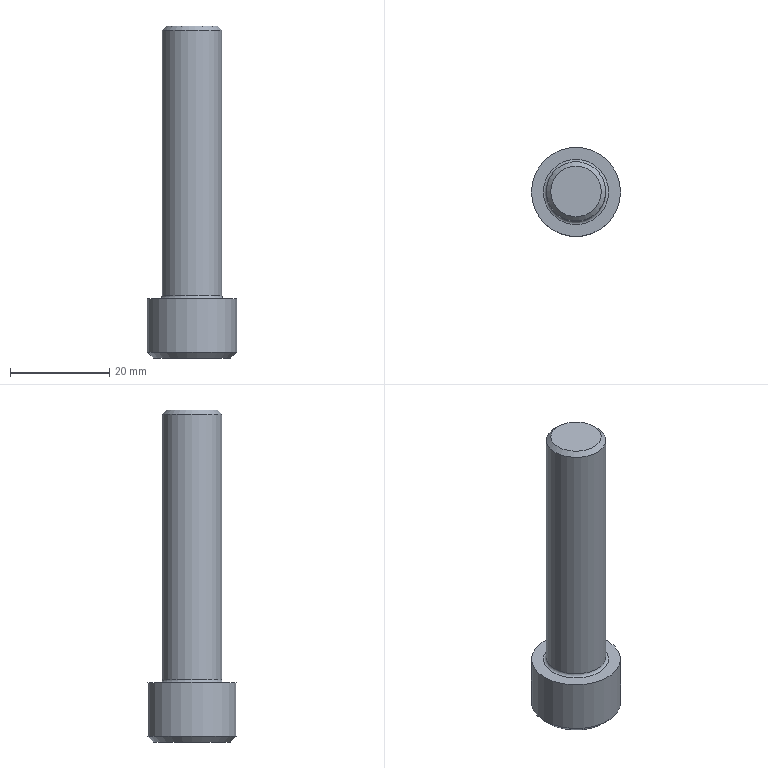Part | STEP file | solid 14 | 1 solid | 21 faces | box 18 x 18 x 67 mm | volume 8702 mm3 | plane 10 | sphere 6 | cylinder 2 | cone 2 | torus 1 | commonest cylinder face diameters 12 x1 18 x1